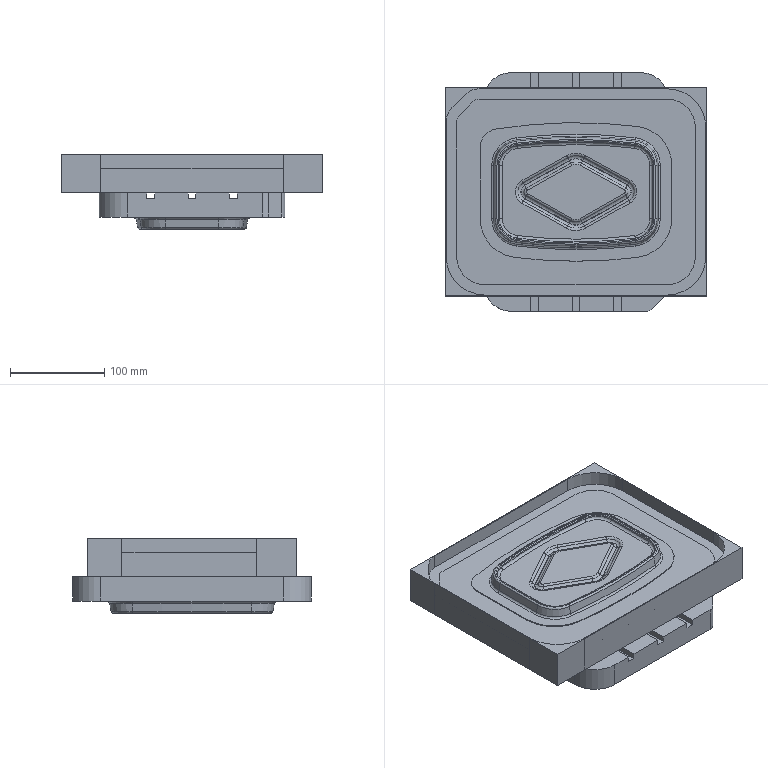NC program | NX | posted with a generic post | part box 278.144 x 254.144 x 79 mm
Lines 1 to 1174 of 124328:
N10 G17 G21 G94 G90
(CAVITY_MILL_1 , TOOL : D16R0.8)
N12 T00 M6
N14 G53
N16 G17 G0 G90 X-26.141 Y101.625 S7000 M3 M8
N18 G43 Z100.5 H0
N20 Z41.5
N22 G94 G1 X0. Z40.13 F4500.
N24 X97.072
N26 G2 X130.025 Y68.672 R32.953
N28 G1 Y-68.672
N30 G2 X97.072 Y-101.625 R32.953
N32 G1 X-97.072
N34 G2 X-130.025 Y-68.672 R32.953
N36 G1 Y74.53
N38 G2 X-126.231 Y83.689 R12.953
N40 G1 X-112.089 Y97.831
N42 G2 X-102.93 Y101.625 R12.953
N44 G1 X0.
N46 Y91.545
N48 X97.072
N50 G2 X119.945 Y68.672 R22.873
N52 G1 Y-68.672
N54 G2 X97.072 Y-91.545 R22.873
N56 G1 X-97.072
N58 G2 X-119.945 Y-68.672 R22.873
N60 G1 Y74.53
N62 G2 X-119.104 Y76.561 R2.873
N64 G1 X-104.961 Y90.703
N66 G2 X-102.93 Y91.545 R2.873
N68 G1 X0.
N70 Y81.465
N72 X97.072
N74 G2 X109.865 Y68.672 R12.793
N76 G1 Y-68.672
N78 G2 X97.072 Y-81.465 R12.793
N80 G1 X-97.072
N82 G2 X-109.865 Y-68.672 R12.793
N84 G1 Y71.544
N86 X-99.945 Y81.465
N88 X0.
N90 Y71.385
N92 X97.072
N94 G2 X99.785 Y68.672 R2.713
N96 G1 Y-68.672
N98 G2 X97.072 Y-71.385 R2.713
N100 G1 X-97.072
N102 G2 X-99.785 Y-68.672 R2.713
N104 G1 Y67.369
N106 X-95.769 Y71.385
N108 X0.
N110 Y61.305
N112 X89.705
N114 Y-61.305
N116 X-89.705
N118 Y61.305
N120 X0.
N122 Y51.225
N124 X79.625
N126 Y-51.225
N128 X-79.625
N130 Y51.225
N132 X0.
N134 Y41.145
N136 X69.545
N138 Y-41.145
N140 X-69.545
N142 Y41.145
N144 X0.
N146 Y31.065
N148 X59.465
N150 Y-31.065
N152 X-59.465
N154 Y31.065
N156 X0.
N158 Y20.985
N160 X49.385
N162 Y-20.985
N164 X-49.385
N166 Y20.985
N168 X0.
N170 Y10.905
N172 X39.305
N174 Y-10.905
N176 X-39.305
N178 Y10.905
N180 X0.
N182 Y0.825
N184 X29.225
N186 Y-0.825
N188 X-29.225
N190 Y0.825
N192 X0.
N194 G3 X3.2 Y4.025 R3.2
N196 G1 Z41.13
N198 G0 Z43.5
N200 X-26.141 Y101.524
N202 Z41.13
N204 G1 X0. Z39.76
N206 X97.072
N208 G2 X129.924 Y68.672 R32.852
N210 G1 Y-68.672
N212 G2 X97.072 Y-101.524 R32.852
N214 G1 X-97.072
N216 G2 X-129.924 Y-68.672 R32.852
N218 G1 Y74.53
N220 G2 X-126.193 Y83.584 R12.852
N222 G1 X-126.16 Y83.618
N224 X-112.046 Y97.731
N226 X-112.008 Y97.769
N228 G2 X-102.93 Y101.524 R12.852
N230 G1 X0.
N232 Y91.444
N234 X97.072
N236 G2 X119.844 Y68.672 R22.772
N238 G1 Y-68.672
N240 G2 X97.072 Y-91.444 R22.772
N242 G1 X-97.072
N244 G2 X-119.844 Y-68.672 R22.772
N246 G1 Y74.53
N248 G2 X-119.025 Y76.497 R2.772
N250 G1 X-104.919 Y90.603
N252 G2 X-102.93 Y91.444 R2.772
N254 G1 X0.
N256 Y81.364
N258 X97.072
N260 G2 X109.764 Y68.672 R12.692
N262 G1 Y-68.673
N264 G2 X97.072 Y-81.364 R12.692
N266 G1 X-97.072
N268 G2 X-109.764 Y-68.672 R12.692
N270 G1 Y71.503
N272 X-99.903 Y81.364
N274 X0.
N276 Y71.284
N278 X97.072
N280 G2 X99.684 Y68.672 R2.612
N282 G1 Y-68.673
N284 G2 X97.072 Y-71.284 R2.612
N286 G1 X-97.072
N288 G2 X-99.684 Y-68.672 R2.612
N290 G1 Y67.327
N292 X-95.728 Y71.284
N294 X0.
N296 Y61.204
N298 X89.604
N300 Y-61.204
N302 X-89.604
N304 Y61.204
N306 X0.
N308 Y51.124
N310 X79.524
N312 Y-51.124
N314 X-79.524
N316 Y51.124
N318 X0.
N320 Y41.044
N322 X69.444
N324 Y-41.044
N326 X-69.444
N328 Y41.044
N330 X0.
N332 Y30.964
N334 X59.364
N336 Y-30.964
N338 X-59.364
N340 Y30.964
N342 X0.
N344 Y20.884
N346 X49.284
N348 Y-20.884
N350 X-49.284
N352 Y20.884
N354 X0.
N356 Y10.804
N358 X39.204
N360 Y-10.804
N362 X-39.204
N364 Y10.804
N366 X0.
N368 Y0.724
N370 X29.124
N372 Y-0.724
N374 X-29.124
N376 Y0.724
N378 X0.
N380 G3 X3.2 Y3.924 R3.2
N382 G1 Z40.76
N384 G0 Z43.13
N386 X-26.141 Y101.522
N388 Z40.76
N390 G1 X0. Z39.39
N392 X97.072
N394 G2 X129.922 Y68.672 R32.85
N396 G1 Y-68.672
N398 G2 X97.072 Y-101.522 R32.85
N400 G1 X-97.072
N402 G2 X-129.922 Y-68.672 R32.85
N404 G1 Y74.53
N406 G2 X-126.158 Y83.616 R12.85
N408 G1 X-112.016 Y97.758
N410 G2 X-102.93 Y101.522 R12.85
N412 G1 X0.
N414 Y91.442
N416 X97.072
N418 G2 X119.842 Y68.672 R22.77
N420 G1 Y-68.672
N422 G2 X97.072 Y-91.442 R22.77
N424 G1 X-97.072
N426 G2 X-119.842 Y-68.672 R22.77
N428 G1 Y74.53
N430 G2 X-119.031 Y76.488 R2.77
N432 G1 X-104.889 Y90.631
N434 G2 X-102.93 Y91.442 R2.77
N436 G1 X0.
N438 Y81.362
N440 X97.072
N442 G2 X109.762 Y68.672 R12.69
N444 G1 Y-68.672
N446 G2 X97.072 Y-81.362 R12.69
N448 G1 X-97.072
N450 G2 X-109.762 Y-68.672 R12.69
N452 G1 Y71.502
N454 X-99.902 Y81.362
N456 X0.
N458 Y71.282
N460 X97.072
N462 G2 X99.682 Y68.672 R2.61
N464 G1 Y-68.672
N466 G2 X97.072 Y-71.282 R2.61
N468 G1 X-97.072
N470 G2 X-99.682 Y-68.672 R2.61
N472 G1 Y67.327
N474 X-95.727 Y71.282
N476 X0.
N478 Y61.202
N480 X89.602
N482 Y-61.202
N484 X-89.602
N486 Y61.202
N488 X0.
N490 Y51.122
N492 X79.522
N494 Y-51.122
N496 X-79.522
N498 Y51.122
N500 X0.
N502 Y41.042
N504 X69.442
N506 Y-41.042
N508 X-69.442
N510 Y41.042
N512 X0.
N514 Y30.962
N516 X59.362
N518 Y-30.962
N520 X-59.362
N522 Y30.962
N524 X0.
N526 Y20.882
N528 X49.282
N530 Y-20.882
N532 X-49.282
N534 Y20.882
N536 X0.
N538 Y10.802
N540 X39.202
N542 Y-10.802
N544 X-39.202
N546 Y10.802
N548 X0.
N550 Y0.722
N552 X29.122
N554 Y-0.722
N556 X-29.122
N558 Y0.722
N560 X0.
N562 G3 X3.2 Y3.922 R3.2
N564 G1 Z40.39
N566 G0 Z42.76
N568 X-26.141 Y101.522
N570 Z40.39
N572 G1 X0. Z39.02
N574 X97.072
N576 G2 X129.922 Y68.672 R32.85
N578 G1 Y-68.672
N580 G2 X97.072 Y-101.522 R32.85
N582 G1 X-97.072
N584 G2 X-129.922 Y-68.672 R32.85
N586 G1 Y74.53
N588 G2 X-126.158 Y83.616 R12.85
N590 G1 X-112.016 Y97.758
N592 G2 X-102.93 Y101.522 R12.85
N594 G1 X0.
N596 Y91.442
N598 X97.072
N600 G2 X119.842 Y68.672 R22.77
N602 G1 Y-68.672
N604 G2 X97.072 Y-91.442 R22.77
N606 G1 X-97.072
N608 G2 X-119.842 Y-68.672 R22.77
N610 G1 Y74.53
N612 G2 X-119.031 Y76.488 R2.77
N614 G1 X-104.889 Y90.631
N616 G2 X-102.93 Y91.442 R2.77
N618 G1 X0.
N620 Y81.362
N622 X97.072
N624 G2 X109.762 Y68.672 R12.69
N626 G1 Y-68.672
N628 G2 X97.072 Y-81.362 R12.69
N630 G1 X-97.072
N632 G2 X-109.762 Y-68.672 R12.69
N634 G1 Y71.502
N636 X-99.902 Y81.362
N638 X0.
N640 Y71.282
N642 X97.072
N644 G2 X99.682 Y68.672 R2.61
N646 G1 Y-68.672
N648 G2 X97.072 Y-71.282 R2.61
N650 G1 X-97.072
N652 G2 X-99.682 Y-68.672 R2.61
N654 G1 Y67.327
N656 X-95.727 Y71.282
N658 X0.
N660 Y61.202
N662 X89.602
N664 Y-61.202
N666 X-89.602
N668 Y61.202
N670 X0.
N672 Y51.122
N674 X79.522
N676 Y-51.122
N678 X-79.522
N680 Y51.122
N682 X0.
N684 Y41.042
N686 X69.442
N688 Y-41.042
N690 X-69.442
N692 Y41.042
N694 X0.
N696 Y30.962
N698 X59.362
N700 Y-30.962
N702 X-59.362
N704 Y30.962
N706 X0.
N708 Y20.882
N710 X49.282
N712 Y-20.882
N714 X-49.282
N716 Y20.882
N718 X0.
N720 Y10.802
N722 X39.202
N724 Y-10.802
N726 X-39.202
N728 Y10.802
N730 X0.
N732 Y0.722
N734 X29.122
N736 Y-0.722
N738 X-29.122
N740 Y0.722
N742 X0.
N744 G3 X3.2 Y3.922 R3.2
N746 G1 Z40.02
N748 G0 Z42.39
N750 X-26.141 Y101.522
N752 Z40.02
N754 G1 X0. Z38.65
N756 X97.072
N758 G2 X129.922 Y68.672 R32.85
N760 G1 Y-68.672
N762 G2 X97.072 Y-101.522 R32.85
N764 G1 X-97.072
N766 G2 X-129.922 Y-68.672 R32.85
N768 G1 Y74.53
N770 G2 X-126.158 Y83.616 R12.85
N772 G1 X-112.016 Y97.758
N774 G2 X-102.93 Y101.522 R12.85
N776 G1 X0.
N778 Y91.442
N780 X97.072
N782 G2 X119.842 Y68.672 R22.77
N784 G1 Y-68.672
N786 G2 X97.072 Y-91.442 R22.77
N788 G1 X-97.072
N790 G2 X-119.842 Y-68.672 R22.77
N792 G1 Y74.53
N794 G2 X-119.031 Y76.488 R2.77
N796 G1 X-104.889 Y90.631
N798 G2 X-102.93 Y91.442 R2.77
N800 G1 X0.
N802 Y81.362
N804 X97.072
N806 G2 X109.762 Y68.672 R12.69
N808 G1 Y-68.672
N810 G2 X97.072 Y-81.362 R12.69
N812 G1 X-97.072
N814 G2 X-109.762 Y-68.672 R12.69
N816 G1 Y71.502
N818 X-99.902 Y81.362
N820 X0.
N822 Y71.282
N824 X97.072
N826 G2 X99.682 Y68.672 R2.61
N828 G1 Y-68.672
N830 G2 X97.072 Y-71.282 R2.61
N832 G1 X-97.072
N834 G2 X-99.682 Y-68.672 R2.61
N836 G1 Y67.327
N838 X-95.727 Y71.282
N840 X0.
N842 Y61.202
N844 X89.602
N846 Y-61.202
N848 X-89.602
N850 Y61.202
N852 X0.
N854 Y51.122
N856 X79.522
N858 Y-51.122
N860 X-79.522
N862 Y51.122
N864 X0.
N866 Y41.042
N868 X69.442
N870 Y-41.042
N872 X-69.442
N874 Y41.042
N876 X0.
N878 Y30.962
N880 X59.362
N882 Y-30.962
N884 X-59.362
N886 Y30.962
N888 X0.
N890 Y20.882
N892 X49.282
N894 Y-20.882
N896 X-49.282
N898 Y20.882
N900 X0.
N902 Y10.802
N904 X39.202
N906 Y-10.802
N908 X-39.202
N910 Y10.802
N912 X0.
N914 Y0.722
N916 X29.122
N918 Y-0.722
N920 X-29.122
N922 Y0.722
N924 X0.
N926 G3 X3.2 Y3.922 R3.2
N928 G1 Z39.65
N930 G0 Z42.02
N932 X-26.268 Y101.522
N934 Z39.65
N936 G1 X0. Z38.273
N938 X97.072
N940 G2 X129.922 Y68.672 R32.85
N942 G1 Y-68.672
N944 G2 X97.072 Y-101.522 R32.85
N946 G1 X-97.072
N948 G2 X-129.922 Y-68.672 R32.85
N950 G1 Y74.53
N952 G2 X-126.158 Y83.616 R12.85
N954 G1 X-112.016 Y97.758
N956 G2 X-102.93 Y101.522 R12.85
N958 G1 X0.
N960 Y91.442
N962 X97.072
N964 G2 X119.842 Y68.672 R22.77
N966 G1 Y-68.672
N968 G2 X97.072 Y-91.442 R22.77
N970 G1 X-97.072
N972 G2 X-119.842 Y-68.672 R22.77
N974 G1 Y74.53
N976 G2 X-119.031 Y76.488 R2.77
N978 G1 X-104.889 Y90.631
N980 G2 X-102.93 Y91.442 R2.77
N982 G1 X0.
N984 Y81.362
N986 X97.072
N988 G2 X109.762 Y68.672 R12.69
N990 G1 Y-68.672
N992 G2 X97.072 Y-81.362 R12.69
N994 G1 X-97.072
N996 G2 X-109.762 Y-68.672 R12.69
N998 G1 Y71.502
N1000 X-99.902 Y81.362
N1002 X0.
N1004 Y71.282
N1006 X97.072
N1008 G2 X99.682 Y68.672 R2.61
N1010 G1 Y46.46
N1012 X89.602
N1014 G3 X70.468 Y61.202 R34.536
N1016 G1 X63.869 Y64.082
N1018 X49.732
N1020 G2 X63.408 Y62.612 R529.229
N1022 X63.869 Y64.082 R7.2
N1024 G1 X70.468 Y61.202
N1026 X89.602
N1028 Y46.46
N1030 X99.682
N1032 Y-68.672
N1034 G2 X97.072 Y-71.282 R2.61
N1036 G1 X70.468
N1038 Y-61.202
N1040 G3 X89.602 Y-46.46 R34.536
N1042 G1 Y-61.202
N1044 X70.468
N1046 X63.408 Y-62.612
N1048 G2 X49.732 Y-64.082 R529.229
N1050 G1 X63.869
N1052 G2 X63.408 Y-62.612 R7.2
N1054 G1 X70.468 Y-61.202
N1056 Y-71.282
N1058 X-97.072
N1060 G2 X-99.682 Y-68.672 R2.61
N1062 G1 Y-46.46
N1064 X-89.602
N1066 G3 X-70.468 Y-61.202 R34.536
N1068 G1 X-63.869 Y-64.082
N1070 X-49.732
N1072 G2 X-63.408 Y-62.612 R529.229
N1074 X-63.869 Y-64.082 R7.2
N1076 G1 X-70.468 Y-61.202
N1078 X-89.602
N1080 Y-46.46
N1082 X-99.682
N1084 Y67.327
N1086 X-95.727 Y71.282
N1088 X-70.468
N1090 Y61.202
N1092 G3 X-89.602 Y46.46 R34.536
N1094 G1 X-87.891 Y45.394
N1096 G2 X-64.251 Y60.478 R32.52
N1098 X64.251 Y60.478 R527.213
N1100 X92.808 Y28.201 R32.52
N1102 G1 Y-28.201
N1104 G2 X64.251 Y-60.478 R32.52
N1106 X-64.251 Y-60.478 R527.213
N1108 X-92.808 Y-28.201 R32.52
N1110 G1 Y28.201
N1112 G2 X-87.891 Y45.394 R32.52
N1114 G1 X-89.602 Y46.46
N1116 Y61.202
N1118 X-70.468
N1120 X-63.408 Y62.612
N1122 G2 X-49.732 Y64.082 R529.229
N1124 G1 X-63.869
N1126 G2 X-63.408 Y62.612 R7.2
N1128 G1 X-70.468 Y61.202
N1130 Y71.282
N1132 X0.
N1134 G3 X3.2 Y74.482 R3.2
N1136 G1 Z39.273
N1138 G0 Z41.65
N1140 X-26.268 Y101.522
N1142 Z39.273
N1144 G1 X0. Z37.897
N1146 X97.072
N1148 G2 X129.922 Y68.672 R32.85
N1150 G1 Y-68.672
N1152 G2 X97.072 Y-101.522 R32.85
N1154 G1 X-97.072
N1156 G2 X-129.922 Y-68.672 R32.85
N1158 G1 Y74.53
N1160 G2 X-126.158 Y83.616 R12.85
N1162 G1 X-112.016 Y97.758
N1164 G2 X-102.93 Y101.522 R12.85
N1166 G1 X0.
N1168 Y91.442
N1170 X97.072
N1172 G2 X119.842 Y68.672 R22.77
N1174 G1 Y-68.672
N1176 G2 X97.072 Y-91.442 R22.77
N1178 G1 X-97.072
N1180 G2 X-119.842 Y-68.672 R22.77
N1182 G1 Y74.53
N1184 G2 X-119.031 Y76.488 R2.77
N1186 G1 X-104.889 Y90.631
N1188 G2 X-102.93 Y91.442 R2.77
N1190 G1 X0.
N1192 Y81.362
N1194 X97.072
N1196 G2 X109.762 Y68.672 R12.69
N1198 G1 Y-68.672
N1200 G2 X97.072 Y-81.362 R12.69
N1202 G1 X-97.072
N1204 G2 X-109.762 Y-68.672 R12.69
N1206 G1 Y71.502
N1208 X-99.902 Y81.362
N1210 X0.
N1212 Y71.282
N1214 X97.072
N1216 G2 X99.682 Y68.672 R2.61
N1218 G1 Y47.436
N1220 X89.602
N1222 G3 X72.129 Y61.202 R35.061
N1224 G1 X65.53 Y64.082
N1226 X55.043
N1228 G2 X64.561 Y63. R529.754
N1230 X65.138 Y62.925 R35.061
N1232 X65.53 Y64.082 R7.2
N1234 G1 X72.129 Y61.202
N1236 X89.602
N1238 Y47.436
N1240 X99.682
N1242 Y-68.672
N1244 G2 X97.072 Y-71.282 R2.61
N1246 G1 X72.129
N1248 Y-61.202
N1250 G3 X89.602 Y-47.436 R35.061
N1252 G1 Y-61.202
N1254 X72.129
N1256 X65.138 Y-62.925
N1258 G2 X64.561 Y-63. R35.061
N1260 X55.043 Y-64.082 R529.754
N1262 G1 X65.53
N1264 G2 X65.138 Y-62.925 R7.2
N1266 G1 X72.129 Y-61.202
N1268 Y-71.282
N1270 X-97.072
N1272 G2 X-99.682 Y-68.672 R2.61
N1274 G1 Y-47.436
N1276 X-89.602
N1278 G3 X-72.129 Y-61.202 R35.061
N1280 G1 X-65.53 Y-64.082
N1282 X-55.043
N1284 G2 X-64.561 Y-63. R529.754
N1286 X-65.138 Y-62.925 R35.061
N1288 X-65.53 Y-64.082 R7.2
N1290 G1 X-72.129 Y-61.202
N1292 X-89.602
N1294 Y-47.436
N1296 X-99.682
N1298 Y67.327
N1300 X-95.727 Y71.282
N1302 X-72.129
N1304 Y61.202
N1306 G3 X-89.602 Y47.436 R35.061
N1308 G1 X-87.917 Y46.33
N1310 G2 X-64.315 Y60.999 R33.045
N1312 X64.315 Y60.999 R527.738
N1314 X93.333 Y28.201 R33.045
N1316 G1 Y-28.201
N1318 G2 X64.315 Y-60.999 R33.045
N1320 X-64.315 Y-60.999 R527.738
N1322 X-93.333 Y-28.201 R33.045
N1324 G1 Y28.201
N1326 G2 X-87.917 Y46.33 R33.045
N1328 G1 X-89.602 Y47.436
N1330 Y61.202
N1332 X-72.129
N1334 X-65.138 Y62.925
N1336 G2 X-64.561 Y63. R35.061
N1338 X-55.043 Y64.082 R529.754
N1340 G1 X-65.53
N1342 G2 X-65.138 Y62.925 R7.2
N1344 G1 X-72.129 Y61.202
N1346 Y71.282
N1348 X0.
N1350 G3 X3.2 Y74.482 R3.2
N1352 G1 Z38.897
N1354 G0 Z41.273
N1356 X-26.268 Y101.522
N1358 Z38.897
N1360 G1 X0. Z37.52
N1362 X97.072
N1364 G2 X129.922 Y68.672 R32.85
N1366 G1 Y-68.672
N1368 G2 X97.072 Y-101.522 R32.85
N1370 G1 X-97.072
N1372 G2 X-129.922 Y-68.672 R32.85
N1374 G1 Y74.53
N1376 G2 X-126.158 Y83.616 R12.85
N1378 G1 X-112.016 Y97.758
N1380 G2 X-102.93 Y101.522 R12.85
N1382 G1 X0.
N1384 Y91.442
N1386 X97.072
N1388 G2 X119.842 Y68.672 R22.77
N1390 G1 Y-68.672
N1392 G2 X97.072 Y-91.442 R22.77
N1394 G1 X-97.072
N1396 G2 X-119.842 Y-68.672 R22.77
N1398 G1 Y74.53
N1400 G2 X-119.031 Y76.488 R2.77
N1402 G1 X-104.889 Y90.631
N1404 G2 X-102.93 Y91.442 R2.77
N1406 G1 X0.
N1408 Y81.362
N1410 X97.072
N1412 G2 X109.762 Y68.672 R12.69
N1414 G1 Y-68.672
N1416 G2 X97.072 Y-81.362 R12.69
N1418 G1 X-97.072
N1420 G2 X-109.762 Y-68.672 R12.69
N1422 G1 Y71.502
N1424 X-99.902 Y81.362
N1426 X0.
N1428 Y71.282
N1430 X97.072
N1432 G2 X99.682 Y68.672 R2.61
N1434 G1 Y48.069
N1436 X89.602
N1438 G3 X73.133 Y61.202 R35.413
N1440 G1 X63.72 Y63.772
N1442 X73.133 Y61.202
N1444 X89.602
N1446 Y48.069
N1448 X99.682
N1450 Y-68.672
N1452 G2 X97.072 Y-71.282 R2.61
N1454 G1 X73.133
N1456 Y-61.202
N1458 G3 X89.602 Y-48.069 R35.413
N1460 G1 Y-61.202
N1462 X73.133
N1464 X63.72 Y-63.772
N1466 X73.133 Y-61.202
N1468 Y-71.282
N1470 X-97.072
N1472 G2 X-99.682 Y-68.672 R2.61
N1474 G1 Y-48.069
N1476 X-89.602
N1478 G3 X-73.133 Y-61.202 R35.413
N1480 G1 X-63.72 Y-63.772
N1482 X-73.133 Y-61.202
N1484 X-89.602
N1486 Y-48.069
N1488 X-99.682
N1490 Y67.327
N1492 X-95.727 Y71.282
N1494 X-73.133
N1496 Y61.202
N1498 G3 X-89.602 Y48.069 R35.413
N1500 G1 X-87.933 Y46.938
N1502 G2 X-64.358 Y61.348 R33.397
N1504 X64.358 Y61.348 R528.09
N1506 X93.685 Y28.201 R33.397
N1508 G1 Y-28.201
N1510 G2 X64.358 Y-61.348 R33.397
N1512 X-64.358 Y-61.348 R528.09
N1514 X-93.685 Y-28.201 R33.397
N1516 G1 Y28.201
N1518 G2 X-87.933 Y46.938 R33.397
N1520 G1 X-89.602 Y48.069
N1522 Y61.202
N1524 X-73.133
N1526 X-63.72 Y63.772
N1528 X-73.133 Y61.202
N1530 Y71.282
N1532 X0.
N1534 G3 X3.2 Y74.482 R3.2
N1536 G1 Z38.52
N1538 G0 Z40.897
N1540 X-26.268 Y101.522
N1542 Z38.52
N1544 G1 X0. Z37.143
N1546 X97.072
N1548 G2 X129.922 Y68.672 R32.85
N1550 G1 Y-68.672
N1552 G2 X97.072 Y-101.522 R32.85
N1554 G1 X-97.072
N1556 G2 X-129.922 Y-68.672 R32.85
N1558 G1 Y74.53
N1560 G2 X-126.158 Y83.616 R12.85
N1562 G1 X-112.016 Y97.758
N1564 G2 X-102.93 Y101.522 R12.85
N1566 G1 X0.
N1568 Y91.442
N1570 X97.072
N1572 G2 X119.842 Y68.672 R22.77
N1574 G1 Y-68.672
N1576 G2 X97.072 Y-91.442 R22.77
N1578 G1 X-97.072
N1580 G2 X-119.842 Y-68.672 R22.77
N1582 G1 Y74.53
N1584 G2 X-119.031 Y76.488 R2.77
N1586 G1 X-104.889 Y90.631
N1588 G2 X-102.93 Y91.442 R2.77
N1590 G1 X0.
N1592 Y81.362
N1594 X97.072
N1596 G2 X109.762 Y68.672 R12.69
N1598 G1 Y-68.672
N1600 G2 X97.072 Y-81.362 R12.69
N1602 G1 X-97.072
N1604 G2 X-109.762 Y-68.672 R12.69
N1606 G1 Y71.502
N1608 X-99.902 Y81.362
N1610 X0.
N1612 Y71.282
N1614 X97.072
N1616 G2 X99.682 Y68.672 R2.61
N1618 G1 Y48.512
N1620 X89.602
N1622 G3 X73.807 Y61.202 R35.663
N1624 G1 X64.94 Y63.818
N1626 X73.807 Y61.202
N1628 X89.602
N1630 Y48.512
N1632 X99.682
N1634 Y-68.672
N1636 G2 X97.072 Y-71.282 R2.61
N1638 G1 X73.807
N1640 Y-61.202
N1642 G3 X89.602 Y-48.512 R35.663
N1644 G1 Y-61.202
N1646 X73.807
N1648 X64.94 Y-63.818
N1650 X73.807 Y-61.202
N1652 Y-71.282
N1654 X-97.072
N1656 G2 X-99.682 Y-68.672 R2.61
N1658 G1 Y-48.512
N1660 X-89.602
N1662 G3 X-73.807 Y-61.202 R35.663
N1664 G1 X-64.94 Y-63.818
N1666 X-73.807 Y-61.202
N1668 X-89.602
N1670 Y-48.512
N1672 X-99.682
N1674 Y67.327
N1676 X-95.727 Y71.282
N1678 X-73.807
N1680 Y61.202
N1682 G3 X-89.602 Y48.512 R35.663
N1684 G1 X-87.945 Y47.363
N1686 G2 X-64.389 Y61.597 R33.647
N1688 X64.389 Y61.597 R528.34
N1690 X93.935 Y28.201 R33.647
N1692 G1 Y-28.201
N1694 G2 X64.389 Y-61.597 R33.647
N1696 X-64.389 Y-61.597 R528.34
N1698 X-93.935 Y-28.201 R33.647
N1700 G1 Y28.201
N1702 G2 X-87.945 Y47.363 R33.647
N1704 G1 X-89.602 Y48.512
N1706 Y61.202
N1708 X-73.807
N1710 X-64.94 Y63.818
N1712 X-73.807 Y61.202
N1714 Y71.282
N1716 X0.
N1718 G3 X3.2 Y74.482 R3.2
N1720 G1 Z38.143
N1722 G0 Z40.52
N1724 X-26.268 Y101.522
N1726 Z38.143
N1728 G1 X0. Z36.767
N1730 X97.072
N1732 G2 X129.922 Y68.672 R32.85
N1734 G1 Y-68.672
N1736 G2 X97.072 Y-101.522 R32.85
N1738 G1 X-97.072
N1740 G2 X-129.922 Y-68.672 R32.85
N1742 G1 Y74.53
N1744 G2 X-126.158 Y83.616 R12.85
N1746 G1 X-112.016 Y97.758
N1748 G2 X-102.93 Y101.522 R12.85
N1750 G1 X0.
N1752 Y91.442
N1754 X97.072
N1756 G2 X119.842 Y68.672 R22.77
N1758 G1 Y-68.672
N1760 G2 X97.072 Y-91.442 R22.77
N1762 G1 X-97.072
N1764 G2 X-119.842 Y-68.672 R22.77
N1766 G1 Y74.53
N1768 G2 X-119.031 Y76.488 R2.77
N1770 G1 X-104.889 Y90.631
N1772 G2 X-102.93 Y91.442 R2.77
N1774 G1 X0.
N1776 Y81.362
N1778 X97.072
N1780 G2 X109.762 Y68.672 R12.69
N1782 G1 Y-68.672
N1784 G2 X97.072 Y-81.362 R12.69
N1786 G1 X-97.072
N1788 G2 X-109.762 Y-68.672 R12.69
N1790 G1 Y71.502
N1792 X-99.902 Y81.362
N1794 X0.
N1796 Y71.282
N1798 X97.072
N1800 G2 X99.682 Y68.672 R2.61
N1802 G1 Y48.82
N1804 X89.602
N1806 G3 X74.266 Y61.202 R35.84
N1808 G1 X65.782 Y63.846
N1810 X74.266 Y61.202
N1812 X89.602
N1814 Y48.82
N1816 X99.682
N1818 Y-68.672
N1820 G2 X97.072 Y-71.282 R2.61
N1822 G1 X74.266
N1824 Y-61.202
N1826 G3 X89.602 Y-48.82 R35.84
N1828 G1 Y-61.202
N1830 X74.266
N1832 X65.782 Y-63.846
N1834 X74.266 Y-61.202
N1836 Y-71.282
N1838 X-97.072
N1840 G2 X-99.682 Y-68.672 R2.61
N1842 G1 Y-48.82
N1844 X-89.602
N1846 G3 X-74.266 Y-61.202 R35.84
N1848 G1 X-65.782 Y-63.846
N1850 X-74.266 Y-61.202
N1852 X-89.602
N1854 Y-48.82
N1856 X-99.682
N1858 Y67.327
N1860 X-95.727 Y71.282
N1862 X-74.266
N1864 Y61.202
N1866 G3 X-89.602 Y48.82 R35.84
N1868 G1 X-87.953 Y47.66
N1870 G2 X-64.41 Y61.772 R33.824
N1872 X64.41 Y61.772 R528.516
N1874 X94.112 Y28.201 R33.824
N1876 G1 Y-28.201
N1878 G2 X64.41 Y-61.772 R33.824
N1880 X-64.41 Y-61.772 R528.516
N1882 X-94.112 Y-28.201 R33.824
N1884 G1 Y28.201
N1886 G2 X-87.953 Y47.66 R33.824
N1888 G1 X-89.602 Y48.82
N1890 Y61.202
N1892 X-74.266
N1894 X-65.782 Y63.846
N1896 X-74.266 Y61.202
N1898 Y71.282
N1900 X0.
N1902 G3 X3.2 Y74.482 R3.2
N1904 G1 Z37.767
N1906 G0 Z40.143
N1908 X-26.268 Y101.522
N1910 Z37.767
N1912 G1 X0. Z36.39
N1914 X97.072
N1916 G2 X129.922 Y68.672 R32.85
N1918 G1 Y-68.672
N1920 G2 X97.072 Y-101.522 R32.85
N1922 G1 X-97.072
N1924 G2 X-129.922 Y-68.672 R32.85
N1926 G1 Y74.53
N1928 G2 X-126.158 Y83.616 R12.85
N1930 G1 X-112.016 Y97.758
N1932 G2 X-102.93 Y101.522 R12.85
N1934 G1 X0.
N1936 Y91.442
N1938 X97.072
N1940 G2 X119.842 Y68.672 R22.77
N1942 G1 Y-68.672
N1944 G2 X97.072 Y-91.442 R22.77
N1946 G1 X-97.072
N1948 G2 X-119.842 Y-68.672 R22.77
N1950 G1 Y74.53
N1952 G2 X-119.031 Y76.488 R2.77
N1954 G1 X-104.889 Y90.631
N1956 G2 X-102.93 Y91.442 R2.77
N1958 G1 X0.
N1960 Y81.362
N1962 X97.072
N1964 G2 X109.762 Y68.672 R12.69
N1966 G1 Y-68.672
N1968 G2 X97.072 Y-81.362 R12.69
N1970 G1 X-97.072
N1972 G2 X-109.762 Y-68.672 R12.69
N1974 G1 Y71.502
N1976 X-99.902 Y81.362
N1978 X0.
N1980 Y71.282
N1982 X97.072
N1984 G2 X99.682 Y68.672 R2.61
N1986 G1 Y49.022
N1988 X89.602
N1990 G3 X74.563 Y61.202 R35.956
N1992 G1 X66.325 Y63.863
N1994 X74.563 Y61.202
N1996 X89.602
N1998 Y49.022
N2000 X99.682
N2002 Y-68.672
N2004 G2 X97.072 Y-71.282 R2.61
N2006 G1 X74.563
N2008 Y-61.202
N2010 G3 X89.602 Y-49.022 R35.956
N2012 G1 Y-61.202
N2014 X74.563
N2016 X66.325 Y-63.863
N2018 X74.563 Y-61.202
N2020 Y-71.282
N2022 X-97.072
N2024 G2 X-99.682 Y-68.672 R2.61
N2026 G1 Y-49.022
N2028 X-89.602
N2030 G3 X-74.563 Y-61.202 R35.956
N2032 G1 X-66.325 Y-63.863
N2034 X-74.563 Y-61.202
N2036 X-89.602
N2038 Y-49.022
N2040 X-99.682
N2042 Y67.327
N2044 X-95.727 Y71.282
N2046 X-74.563
N2048 Y61.202
N2050 G3 X-89.602 Y49.022 R35.956
N2052 G1 X-87.959 Y47.855
N2054 G2 X-64.425 Y61.888 R33.94
N2056 X64.425 Y61.888 R528.633
N2058 X94.229 Y28.201 R33.94
N2060 G1 Y-28.201
N2062 G2 X64.425 Y-61.888 R33.94
N2064 X-64.425 Y-61.888 R528.633
N2066 X-94.229 Y-28.201 R33.94
N2068 G1 Y28.201
N2070 G2 X-87.959 Y47.855 R33.94
N2072 G1 X-89.602 Y49.022
N2074 Y61.202
N2076 X-74.563
N2078 X-66.325 Y63.863
N2080 X-74.563 Y61.202
N2082 Y71.282
N2084 X0.
N2086 G3 X3.2 Y74.482 R3.2
N2088 G1 Z37.39
N2090 G0 Z39.767
N2092 X-26.268 Y101.522
N2094 Z37.39
N2096 G1 X0. Z36.014
N2098 X97.072
N2100 G2 X129.922 Y68.672 R32.85
N2102 G1 Y-68.672
N2104 G2 X97.072 Y-101.522 R32.85
N2106 G1 X-97.072
N2108 G2 X-129.922 Y-68.672 R32.85
N2110 G1 Y74.53
N2112 G2 X-126.158 Y83.616 R12.85
N2114 G1 X-112.016 Y97.758
N2116 G2 X-102.93 Y101.522 R12.85
N2118 G1 X0.
N2120 Y91.442
N2122 X97.072
N2124 G2 X119.842 Y68.672 R22.77
N2126 G1 Y-68.672
N2128 G2 X97.072 Y-91.442 R22.77
N2130 G1 X-97.072
N2132 G2 X-119.842 Y-68.672 R22.77
N2134 G1 Y74.53
N2136 G2 X-119.031 Y76.488 R2.77
N2138 G1 X-104.889 Y90.631
N2140 G2 X-102.93 Y91.442 R2.77
N2142 G1 X0.
N2144 Y81.362
N2146 X97.072
N2148 G2 X109.762 Y68.672 R12.69
N2150 G1 Y-68.672
N2152 G2 X97.072 Y-81.362 R12.69
N2154 G1 X-97.072
N2156 G2 X-109.762 Y-68.672 R12.69
N2158 G1 Y71.502
N2160 X-99.902 Y81.362
N2162 X0.
N2164 Y71.282
N2166 X97.072
N2168 G2 X99.682 Y68.672 R2.61
N2170 G1 Y49.146
N2172 X89.602
N2174 G3 X74.742 Y61.202 R36.028
N2176 G1 X66.65 Y63.872
N2178 X74.742 Y61.202
N2180 X89.602
N2182 Y49.146
N2184 X99.682
N2186 Y-68.672
N2188 G2 X97.072 Y-71.282 R2.61
N2190 G1 X74.742
N2192 Y-61.202
N2194 G3 X89.602 Y-49.146 R36.028
N2196 G1 Y-61.202
N2198 X74.742
N2200 X66.65 Y-63.872
N2202 X74.742 Y-61.202
N2204 Y-71.282
N2206 X-97.072
N2208 G2 X-99.682 Y-68.672 R2.61
N2210 G1 Y-49.146
N2212 X-89.602
N2214 G3 X-74.742 Y-61.202 R36.028
N2216 G1 X-66.65 Y-63.872
N2218 X-74.742 Y-61.202
N2220 X-89.602
N2222 Y-49.146
N2224 X-99.682
N2226 Y67.327
N2228 X-95.727 Y71.282
N2230 X-74.742
N2232 Y61.202
N2234 G3 X-89.602 Y49.146 R36.028
N2236 G1 X-87.962 Y47.974
N2238 G2 X-64.433 Y61.959 R34.012
N2240 X64.433 Y61.959 R528.705
N2242 X94.3 Y28.201 R34.012
N2244 G1 Y-28.201
N2246 G2 X64.433 Y-61.959 R34.012
N2248 X-64.433 Y-61.959 R528.705
N2250 X-94.3 Y-28.201 R34.012
N2252 G1 Y28.201
N2254 G2 X-87.962 Y47.974 R34.012
N2256 G1 X-89.602 Y49.146
N2258 Y61.202
N2260 X-74.742
N2262 X-66.65 Y63.872
N2264 X-74.742 Y61.202
N2266 Y71.282
N2268 X0.
N2270 G3 X3.2 Y74.482 R3.2
N2272 G1 Z37.014
N2274 G0 Z39.39
N2276 X-26.268 Y101.522
N2278 Z37.014
N2280 G1 X0. Z35.637
N2282 X97.072
N2284 G2 X129.922 Y68.672 R32.85
N2286 G1 Y-68.672
N2288 G2 X97.072 Y-101.522 R32.85
N2290 G1 X-97.072
N2292 G2 X-129.922 Y-68.672 R32.85
N2294 G1 Y74.53
N2296 G2 X-126.158 Y83.616 R12.85
N2298 G1 X-112.016 Y97.758
N2300 G2 X-102.93 Y101.522 R12.85
N2302 G1 X0.
N2304 Y91.442
N2306 X97.072
N2308 G2 X119.842 Y68.672 R22.77
N2310 G1 Y-68.672
N2312 G2 X97.072 Y-91.442 R22.77
N2314 G1 X-97.072
N2316 G2 X-119.842 Y-68.672 R22.77
N2318 G1 Y74.53
N2320 G2 X-119.031 Y76.488 R2.77
N2322 G1 X-104.889 Y90.631
N2324 G2 X-102.93 Y91.442 R2.77
N2326 G1 X0.
N2328 Y81.362
N2330 X97.072
N2332 G2 X109.762 Y68.672 R12.69
N2334 G1 Y-68.672
N2336 G2 X97.072 Y-81.362 R12.69
N2338 G1 X-97.072
N2340 G2 X-109.762 Y-68.672 R12.69
N2342 G1 Y71.502
N2344 X-99.902 Y81.362
N2346 X0.